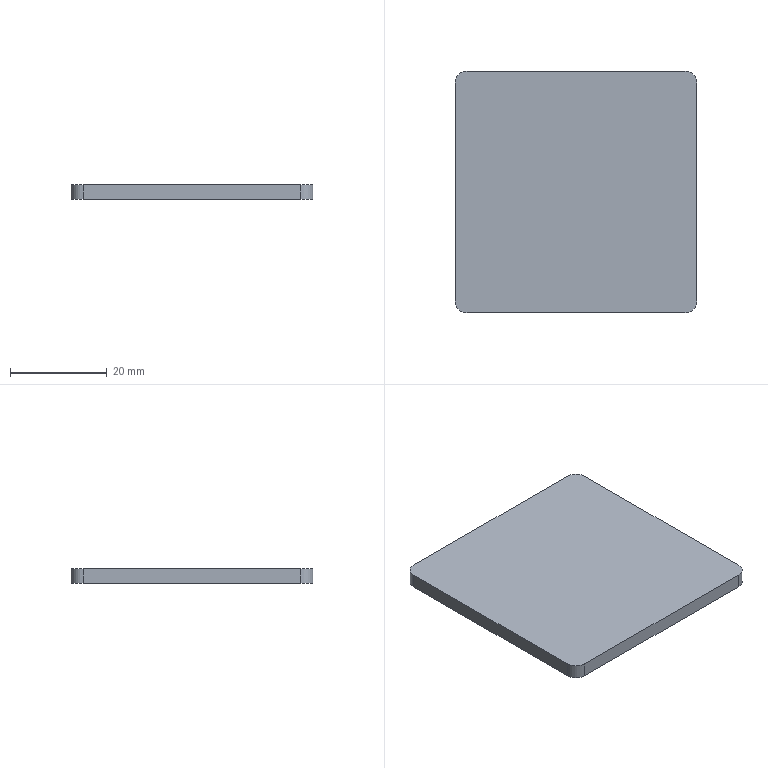Part | STEP file | 6100518 | 1 solid | 10 faces | box 50 x 50 x 3 mm | volume 7484 mm3 | plane 6 | cylinder 4 | commonest cylinder face diameters 5 x4
STEP:
#1=CARTESIAN_POINT('',(0.,0.,0.));
#2=DIRECTION('',(0.,0.,1.));
#3=DIRECTION('',(1.,0.,0.));
#4=AXIS2_PLACEMENT_3D('',#1,#2,#3);
#5=CARTESIAN_POINT('',(22.5,-25.,0.));
#6=VERTEX_POINT('',#5);
#7=CARTESIAN_POINT('',(25.,-22.5,0.));
#8=VERTEX_POINT('',#7);
#9=CARTESIAN_POINT('',(22.5,-22.5,0.));
#10=DIRECTION('',(0.,0.,1.));
#11=DIRECTION('',(1.,0.,0.));
#12=AXIS2_PLACEMENT_3D('',#9,#10,#11);
#13=CIRCLE('',#12,2.5);
#14=CARTESIAN_POINT('',(22.5,-22.5,3.));
#15=DIRECTION('',(0.,0.,-1.));
#16=DIRECTION('',(-1.,0.,0.));
#17=AXIS2_PLACEMENT_3D('',#14,#15,#16);
#18=CYLINDRICAL_SURFACE('',#17,2.5);
#19=CARTESIAN_POINT('',(9.425,3.));
#20=DIRECTION('',(-1.,0.));
#21=VECTOR('',#20,1.);
#22=LINE('',#19,#21);
#23=(GEOMETRIC_REPRESENTATION_CONTEXT(2)PARAMETRIC_REPRESENTATION_CONTEXT()REPRESENTATION_CONTEXT('',''));
#24=DEFINITIONAL_REPRESENTATION('',(#22),#23);
#25=PCURVE('',#18,#24);
#26=CARTESIAN_POINT('',(22.5,-22.5,0.));
#27=DIRECTION('',(0.,0.,1.));
#28=DIRECTION('',(1.,0.,0.));
#29=AXIS2_PLACEMENT_3D('',#26,#27,#28);
#30=PLANE('',#29);
#31=CARTESIAN_POINT('',(0.,0.));
#32=DIRECTION('',(1.,0.));
#33=AXIS2_PLACEMENT_2D('',#31,#32);
#34=CIRCLE('',#33,2.5);
#35=(GEOMETRIC_REPRESENTATION_CONTEXT(2)PARAMETRIC_REPRESENTATION_CONTEXT()REPRESENTATION_CONTEXT('',''));
#36=DEFINITIONAL_REPRESENTATION('',(#34),#35);
#37=PCURVE('',#30,#36);
#38=SURFACE_CURVE('',#13,(#25,#37),.PCURVE_S1.);
#39=EDGE_CURVE('',#6,#8,#38,.T.);
#40=ORIENTED_EDGE('',*,*,#39,.T.);
#41=CARTESIAN_POINT('',(25.,-22.5,3.));
#42=VERTEX_POINT('',#41);
#43=CARTESIAN_POINT('',(25.,-22.5,3.));
#44=DIRECTION('',(0.,0.,-1.));
#45=VECTOR('',#44,1.);
#46=LINE('',#43,#45);
#47=CARTESIAN_POINT('',(3.142,0.));
#48=DIRECTION('',(0.,1.));
#49=VECTOR('',#48,1.);
#50=LINE('',#47,#49);
#51=(GEOMETRIC_REPRESENTATION_CONTEXT(2)PARAMETRIC_REPRESENTATION_CONTEXT()REPRESENTATION_CONTEXT('',''));
#52=DEFINITIONAL_REPRESENTATION('',(#50),#51);
#53=PCURVE('',#18,#52);
#54=CARTESIAN_POINT('',(25.,22.5,3.));
#55=DIRECTION('',(-1.,0.,0.));
#56=DIRECTION('',(0.,-1.,0.));
#57=AXIS2_PLACEMENT_3D('',#54,#55,#56);
#58=PLANE('',#57);
#59=CARTESIAN_POINT('',(45.,0.));
#60=DIRECTION('',(0.,-1.));
#61=VECTOR('',#60,1.);
#62=LINE('',#59,#61);
#63=(GEOMETRIC_REPRESENTATION_CONTEXT(2)PARAMETRIC_REPRESENTATION_CONTEXT()REPRESENTATION_CONTEXT('',''));
#64=DEFINITIONAL_REPRESENTATION('',(#62),#63);
#65=PCURVE('',#58,#64);
#66=SURFACE_CURVE('',#46,(#53,#65),.PCURVE_S1.);
#67=EDGE_CURVE('',#42,#8,#66,.T.);
#68=ORIENTED_EDGE('',*,*,#67,.F.);
#69=CARTESIAN_POINT('',(22.5,-25.,3.));
#70=VERTEX_POINT('',#69);
#71=CARTESIAN_POINT('',(22.5,-22.5,3.));
#72=DIRECTION('',(0.,0.,1.));
#73=DIRECTION('',(1.,0.,0.));
#74=AXIS2_PLACEMENT_3D('',#71,#72,#73);
#75=CIRCLE('',#74,2.5);
#76=CARTESIAN_POINT('',(9.425,0.));
#77=DIRECTION('',(-1.,0.));
#78=VECTOR('',#77,1.);
#79=LINE('',#76,#78);
#80=(GEOMETRIC_REPRESENTATION_CONTEXT(2)PARAMETRIC_REPRESENTATION_CONTEXT()REPRESENTATION_CONTEXT('',''));
#81=DEFINITIONAL_REPRESENTATION('',(#79),#80);
#82=PCURVE('',#18,#81);
#83=CARTESIAN_POINT('',(22.5,-22.5,3.));
#84=DIRECTION('',(0.,0.,1.));
#85=DIRECTION('',(1.,0.,0.));
#86=AXIS2_PLACEMENT_3D('',#83,#84,#85);
#87=PLANE('',#86);
#88=CARTESIAN_POINT('',(0.,0.));
#89=DIRECTION('',(1.,0.));
#90=AXIS2_PLACEMENT_2D('',#88,#89);
#91=CIRCLE('',#90,2.5);
#92=(GEOMETRIC_REPRESENTATION_CONTEXT(2)PARAMETRIC_REPRESENTATION_CONTEXT()REPRESENTATION_CONTEXT('',''));
#93=DEFINITIONAL_REPRESENTATION('',(#91),#92);
#94=PCURVE('',#87,#93);
#95=SURFACE_CURVE('',#75,(#82,#94),.PCURVE_S1.);
#96=EDGE_CURVE('',#70,#42,#95,.T.);
#97=ORIENTED_EDGE('',*,*,#96,.F.);
#98=CARTESIAN_POINT('',(22.5,-25.,3.));
#99=DIRECTION('',(0.,0.,-1.));
#100=VECTOR('',#99,1.);
#101=LINE('',#98,#100);
#102=CARTESIAN_POINT('',(4.712,0.));
#103=DIRECTION('',(0.,1.));
#104=VECTOR('',#103,1.);
#105=LINE('',#102,#104);
#106=(GEOMETRIC_REPRESENTATION_CONTEXT(2)PARAMETRIC_REPRESENTATION_CONTEXT()REPRESENTATION_CONTEXT('',''));
#107=DEFINITIONAL_REPRESENTATION('',(#105),#106);
#108=PCURVE('',#18,#107);
#109=CARTESIAN_POINT('',(-22.5,-25.,3.));
#110=DIRECTION('',(0.,1.,0.));
#111=DIRECTION('',(-1.,0.,0.));
#112=AXIS2_PLACEMENT_3D('',#109,#110,#111);
#113=PLANE('',#112);
#114=CARTESIAN_POINT('',(-45.,0.));
#115=DIRECTION('',(0.,-1.));
#116=VECTOR('',#115,1.);
#117=LINE('',#114,#116);
#118=(GEOMETRIC_REPRESENTATION_CONTEXT(2)PARAMETRIC_REPRESENTATION_CONTEXT()REPRESENTATION_CONTEXT('',''));
#119=DEFINITIONAL_REPRESENTATION('',(#117),#118);
#120=PCURVE('',#113,#119);
#121=SURFACE_CURVE('',#101,(#108,#120),.PCURVE_S1.);
#122=EDGE_CURVE('',#70,#6,#121,.T.);
#123=ORIENTED_EDGE('',*,*,#122,.T.);
#124=EDGE_LOOP('',(#40,#68,#97,#123));
#125=FACE_BOUND('',#124,.T.);
#126=ADVANCED_FACE('',(#125),#18,.T.);
#127=CARTESIAN_POINT('',(25.,22.5,0.));
#128=VERTEX_POINT('',#127);
#129=CARTESIAN_POINT('',(25.,22.5,0.));
#130=DIRECTION('',(0.,1.,0.));
#131=VECTOR('',#130,1.);
#132=LINE('',#129,#131);
#133=CARTESIAN_POINT('',(0.,-3.));
#134=DIRECTION('',(-1.,0.));
#135=VECTOR('',#134,1.);
#136=LINE('',#133,#135);
#137=(GEOMETRIC_REPRESENTATION_CONTEXT(2)PARAMETRIC_REPRESENTATION_CONTEXT()REPRESENTATION_CONTEXT('',''));
#138=DEFINITIONAL_REPRESENTATION('',(#136),#137);
#139=PCURVE('',#58,#138);
#140=CARTESIAN_POINT('',(2.5,45.));
#141=DIRECTION('',(0.,1.));
#142=VECTOR('',#141,1.);
#143=LINE('',#140,#142);
#144=(GEOMETRIC_REPRESENTATION_CONTEXT(2)PARAMETRIC_REPRESENTATION_CONTEXT()REPRESENTATION_CONTEXT('',''));
#145=DEFINITIONAL_REPRESENTATION('',(#143),#144);
#146=PCURVE('',#30,#145);
#147=SURFACE_CURVE('',#132,(#139,#146),.PCURVE_S1.);
#148=EDGE_CURVE('',#8,#128,#147,.T.);
#149=ORIENTED_EDGE('',*,*,#148,.T.);
#150=CARTESIAN_POINT('',(25.,22.5,3.));
#151=VERTEX_POINT('',#150);
#152=CARTESIAN_POINT('',(25.,22.5,3.));
#153=DIRECTION('',(0.,0.,-1.));
#154=VECTOR('',#153,1.);
#155=LINE('',#152,#154);
#156=CARTESIAN_POINT('',(0.,0.));
#157=DIRECTION('',(0.,-1.));
#158=VECTOR('',#157,1.);
#159=LINE('',#156,#158);
#160=(GEOMETRIC_REPRESENTATION_CONTEXT(2)PARAMETRIC_REPRESENTATION_CONTEXT()REPRESENTATION_CONTEXT('',''));
#161=DEFINITIONAL_REPRESENTATION('',(#159),#160);
#162=PCURVE('',#58,#161);
#163=CARTESIAN_POINT('',(22.5,22.5,3.));
#164=DIRECTION('',(0.,0.,-1.));
#165=DIRECTION('',(-1.,0.,0.));
#166=AXIS2_PLACEMENT_3D('',#163,#164,#165);
#167=CYLINDRICAL_SURFACE('',#166,2.5);
#168=CARTESIAN_POINT('',(3.142,0.));
#169=DIRECTION('',(0.,1.));
#170=VECTOR('',#169,1.);
#171=LINE('',#168,#170);
#172=(GEOMETRIC_REPRESENTATION_CONTEXT(2)PARAMETRIC_REPRESENTATION_CONTEXT()REPRESENTATION_CONTEXT('',''));
#173=DEFINITIONAL_REPRESENTATION('',(#171),#172);
#174=PCURVE('',#167,#173);
#175=SURFACE_CURVE('',#155,(#162,#174),.PCURVE_S1.);
#176=EDGE_CURVE('',#151,#128,#175,.T.);
#177=ORIENTED_EDGE('',*,*,#176,.F.);
#178=CARTESIAN_POINT('',(25.,22.5,3.));
#179=DIRECTION('',(0.,1.,0.));
#180=VECTOR('',#179,1.);
#181=LINE('',#178,#180);
#182=CARTESIAN_POINT('',(0.,0.));
#183=DIRECTION('',(-1.,0.));
#184=VECTOR('',#183,1.);
#185=LINE('',#182,#184);
#186=(GEOMETRIC_REPRESENTATION_CONTEXT(2)PARAMETRIC_REPRESENTATION_CONTEXT()REPRESENTATION_CONTEXT('',''));
#187=DEFINITIONAL_REPRESENTATION('',(#185),#186);
#188=PCURVE('',#58,#187);
#189=CARTESIAN_POINT('',(2.5,45.));
#190=DIRECTION('',(0.,1.));
#191=VECTOR('',#190,1.);
#192=LINE('',#189,#191);
#193=(GEOMETRIC_REPRESENTATION_CONTEXT(2)PARAMETRIC_REPRESENTATION_CONTEXT()REPRESENTATION_CONTEXT('',''));
#194=DEFINITIONAL_REPRESENTATION('',(#192),#193);
#195=PCURVE('',#87,#194);
#196=SURFACE_CURVE('',#181,(#188,#195),.PCURVE_S1.);
#197=EDGE_CURVE('',#42,#151,#196,.T.);
#198=ORIENTED_EDGE('',*,*,#197,.F.);
#199=ORIENTED_EDGE('',*,*,#67,.T.);
#200=EDGE_LOOP('',(#149,#177,#198,#199));
#201=FACE_BOUND('',#200,.T.);
#202=ADVANCED_FACE('',(#201),#58,.F.);
#203=CARTESIAN_POINT('',(22.5,25.,0.));
#204=VERTEX_POINT('',#203);
#205=CARTESIAN_POINT('',(22.5,22.5,0.));
#206=DIRECTION('',(0.,0.,1.));
#207=DIRECTION('',(-1.,0.,0.));
#208=AXIS2_PLACEMENT_3D('',#205,#206,#207);
#209=CIRCLE('',#208,2.5);
#210=CARTESIAN_POINT('',(6.283,3.));
#211=DIRECTION('',(-1.,0.));
#212=VECTOR('',#211,1.);
#213=LINE('',#210,#212);
#214=(GEOMETRIC_REPRESENTATION_CONTEXT(2)PARAMETRIC_REPRESENTATION_CONTEXT()REPRESENTATION_CONTEXT('',''));
#215=DEFINITIONAL_REPRESENTATION('',(#213),#214);
#216=PCURVE('',#167,#215);
#217=CARTESIAN_POINT('',(0.,45.));
#218=DIRECTION('',(-1.,0.));
#219=AXIS2_PLACEMENT_2D('',#217,#218);
#220=CIRCLE('',#219,2.5);
#221=(GEOMETRIC_REPRESENTATION_CONTEXT(2)PARAMETRIC_REPRESENTATION_CONTEXT()REPRESENTATION_CONTEXT('',''));
#222=DEFINITIONAL_REPRESENTATION('',(#220),#221);
#223=PCURVE('',#30,#222);
#224=SURFACE_CURVE('',#209,(#216,#223),.PCURVE_S1.);
#225=EDGE_CURVE('',#128,#204,#224,.T.);
#226=ORIENTED_EDGE('',*,*,#225,.T.);
#227=CARTESIAN_POINT('',(22.5,25.,3.));
#228=VERTEX_POINT('',#227);
#229=CARTESIAN_POINT('',(22.5,25.,3.));
#230=DIRECTION('',(0.,0.,-1.));
#231=VECTOR('',#230,1.);
#232=LINE('',#229,#231);
#233=CARTESIAN_POINT('',(1.571,0.));
#234=DIRECTION('',(0.,1.));
#235=VECTOR('',#234,1.);
#236=LINE('',#233,#235);
#237=(GEOMETRIC_REPRESENTATION_CONTEXT(2)PARAMETRIC_REPRESENTATION_CONTEXT()REPRESENTATION_CONTEXT('',''));
#238=DEFINITIONAL_REPRESENTATION('',(#236),#237);
#239=PCURVE('',#167,#238);
#240=CARTESIAN_POINT('',(-22.5,25.,3.));
#241=DIRECTION('',(0.,-1.,0.));
#242=DIRECTION('',(0.,0.,-1.));
#243=AXIS2_PLACEMENT_3D('',#240,#241,#242);
#244=PLANE('',#243);
#245=CARTESIAN_POINT('',(0.,45.));
#246=DIRECTION('',(1.,0.));
#247=VECTOR('',#246,1.);
#248=LINE('',#245,#247);
#249=(GEOMETRIC_REPRESENTATION_CONTEXT(2)PARAMETRIC_REPRESENTATION_CONTEXT()REPRESENTATION_CONTEXT('',''));
#250=DEFINITIONAL_REPRESENTATION('',(#248),#249);
#251=PCURVE('',#244,#250);
#252=SURFACE_CURVE('',#232,(#239,#251),.PCURVE_S1.);
#253=EDGE_CURVE('',#228,#204,#252,.T.);
#254=ORIENTED_EDGE('',*,*,#253,.F.);
#255=CARTESIAN_POINT('',(22.5,22.5,3.));
#256=DIRECTION('',(0.,0.,1.));
#257=DIRECTION('',(-1.,0.,0.));
#258=AXIS2_PLACEMENT_3D('',#255,#256,#257);
#259=CIRCLE('',#258,2.5);
#260=CARTESIAN_POINT('',(6.283,0.));
#261=DIRECTION('',(-1.,0.));
#262=VECTOR('',#261,1.);
#263=LINE('',#260,#262);
#264=(GEOMETRIC_REPRESENTATION_CONTEXT(2)PARAMETRIC_REPRESENTATION_CONTEXT()REPRESENTATION_CONTEXT('',''));
#265=DEFINITIONAL_REPRESENTATION('',(#263),#264);
#266=PCURVE('',#167,#265);
#267=CARTESIAN_POINT('',(0.,45.));
#268=DIRECTION('',(-1.,0.));
#269=AXIS2_PLACEMENT_2D('',#267,#268);
#270=CIRCLE('',#269,2.5);
#271=(GEOMETRIC_REPRESENTATION_CONTEXT(2)PARAMETRIC_REPRESENTATION_CONTEXT()REPRESENTATION_CONTEXT('',''));
#272=DEFINITIONAL_REPRESENTATION('',(#270),#271);
#273=PCURVE('',#87,#272);
#274=SURFACE_CURVE('',#259,(#266,#273),.PCURVE_S1.);
#275=EDGE_CURVE('',#151,#228,#274,.T.);
#276=ORIENTED_EDGE('',*,*,#275,.F.);
#277=ORIENTED_EDGE('',*,*,#176,.T.);
#278=EDGE_LOOP('',(#226,#254,#276,#277));
#279=FACE_BOUND('',#278,.T.);
#280=ADVANCED_FACE('',(#279),#167,.T.);
#281=CARTESIAN_POINT('',(-22.5,25.,0.));
#282=VERTEX_POINT('',#281);
#283=CARTESIAN_POINT('',(-22.5,25.,0.));
#284=DIRECTION('',(-1.,0.,0.));
#285=VECTOR('',#284,1.);
#286=LINE('',#283,#285);
#287=CARTESIAN_POINT('',(3.,0.));
#288=DIRECTION('',(0.,-1.));
#289=VECTOR('',#288,1.);
#290=LINE('',#287,#289);
#291=(GEOMETRIC_REPRESENTATION_CONTEXT(2)PARAMETRIC_REPRESENTATION_CONTEXT()REPRESENTATION_CONTEXT('',''));
#292=DEFINITIONAL_REPRESENTATION('',(#290),#291);
#293=PCURVE('',#244,#292);
#294=CARTESIAN_POINT('',(-45.,47.5));
#295=DIRECTION('',(-1.,0.));
#296=VECTOR('',#295,1.);
#297=LINE('',#294,#296);
#298=(GEOMETRIC_REPRESENTATION_CONTEXT(2)PARAMETRIC_REPRESENTATION_CONTEXT()REPRESENTATION_CONTEXT('',''));
#299=DEFINITIONAL_REPRESENTATION('',(#297),#298);
#300=PCURVE('',#30,#299);
#301=SURFACE_CURVE('',#286,(#293,#300),.PCURVE_S1.);
#302=EDGE_CURVE('',#204,#282,#301,.T.);
#303=ORIENTED_EDGE('',*,*,#302,.T.);
#304=CARTESIAN_POINT('',(-22.5,25.,3.));
#305=VERTEX_POINT('',#304);
#306=CARTESIAN_POINT('',(-22.5,25.,3.));
#307=DIRECTION('',(0.,0.,-1.));
#308=VECTOR('',#307,1.);
#309=LINE('',#306,#308);
#310=CARTESIAN_POINT('',(0.,0.));
#311=DIRECTION('',(1.,0.));
#312=VECTOR('',#311,1.);
#313=LINE('',#310,#312);
#314=(GEOMETRIC_REPRESENTATION_CONTEXT(2)PARAMETRIC_REPRESENTATION_CONTEXT()REPRESENTATION_CONTEXT('',''));
#315=DEFINITIONAL_REPRESENTATION('',(#313),#314);
#316=PCURVE('',#244,#315);
#317=CARTESIAN_POINT('',(-22.5,22.5,3.));
#318=DIRECTION('',(0.,0.,-1.));
#319=DIRECTION('',(-1.,0.,0.));
#320=AXIS2_PLACEMENT_3D('',#317,#318,#319);
#321=CYLINDRICAL_SURFACE('',#320,2.5);
#322=CARTESIAN_POINT('',(1.571,0.));
#323=DIRECTION('',(0.,1.));
#324=VECTOR('',#323,1.);
#325=LINE('',#322,#324);
#326=(GEOMETRIC_REPRESENTATION_CONTEXT(2)PARAMETRIC_REPRESENTATION_CONTEXT()REPRESENTATION_CONTEXT('',''));
#327=DEFINITIONAL_REPRESENTATION('',(#325),#326);
#328=PCURVE('',#321,#327);
#329=SURFACE_CURVE('',#309,(#316,#328),.PCURVE_S1.);
#330=EDGE_CURVE('',#305,#282,#329,.T.);
#331=ORIENTED_EDGE('',*,*,#330,.F.);
#332=CARTESIAN_POINT('',(-22.5,25.,3.));
#333=DIRECTION('',(-1.,0.,0.));
#334=VECTOR('',#333,1.);
#335=LINE('',#332,#334);
#336=CARTESIAN_POINT('',(0.,0.));
#337=DIRECTION('',(0.,-1.));
#338=VECTOR('',#337,1.);
#339=LINE('',#336,#338);
#340=(GEOMETRIC_REPRESENTATION_CONTEXT(2)PARAMETRIC_REPRESENTATION_CONTEXT()REPRESENTATION_CONTEXT('',''));
#341=DEFINITIONAL_REPRESENTATION('',(#339),#340);
#342=PCURVE('',#244,#341);
#343=CARTESIAN_POINT('',(-45.,47.5));
#344=DIRECTION('',(-1.,0.));
#345=VECTOR('',#344,1.);
#346=LINE('',#343,#345);
#347=(GEOMETRIC_REPRESENTATION_CONTEXT(2)PARAMETRIC_REPRESENTATION_CONTEXT()REPRESENTATION_CONTEXT('',''));
#348=DEFINITIONAL_REPRESENTATION('',(#346),#347);
#349=PCURVE('',#87,#348);
#350=SURFACE_CURVE('',#335,(#342,#349),.PCURVE_S1.);
#351=EDGE_CURVE('',#228,#305,#350,.T.);
#352=ORIENTED_EDGE('',*,*,#351,.F.);
#353=ORIENTED_EDGE('',*,*,#253,.T.);
#354=EDGE_LOOP('',(#303,#331,#352,#353));
#355=FACE_BOUND('',#354,.T.);
#356=ADVANCED_FACE('',(#355),#244,.F.);
#357=CARTESIAN_POINT('',(-25.,22.5,0.));
#358=VERTEX_POINT('',#357);
#359=CARTESIAN_POINT('',(-22.5,22.5,0.));
#360=DIRECTION('',(0.,0.,1.));
#361=DIRECTION('',(1.,0.,0.));
#362=AXIS2_PLACEMENT_3D('',#359,#360,#361);
#363=CIRCLE('',#362,2.5);
#364=CARTESIAN_POINT('',(3.142,3.));
#365=DIRECTION('',(-1.,0.));
#366=VECTOR('',#365,1.);
#367=LINE('',#364,#366);
#368=(GEOMETRIC_REPRESENTATION_CONTEXT(2)PARAMETRIC_REPRESENTATION_CONTEXT()REPRESENTATION_CONTEXT('',''));
#369=DEFINITIONAL_REPRESENTATION('',(#367),#368);
#370=PCURVE('',#321,#369);
#371=CARTESIAN_POINT('',(-45.,45.));
#372=DIRECTION('',(1.,0.));
#373=AXIS2_PLACEMENT_2D('',#371,#372);
#374=CIRCLE('',#373,2.5);
#375=(GEOMETRIC_REPRESENTATION_CONTEXT(2)PARAMETRIC_REPRESENTATION_CONTEXT()REPRESENTATION_CONTEXT('',''));
#376=DEFINITIONAL_REPRESENTATION('',(#374),#375);
#377=PCURVE('',#30,#376);
#378=SURFACE_CURVE('',#363,(#370,#377),.PCURVE_S1.);
#379=EDGE_CURVE('',#282,#358,#378,.T.);
#380=ORIENTED_EDGE('',*,*,#379,.T.);
#381=CARTESIAN_POINT('',(-25.,22.5,3.));
#382=VERTEX_POINT('',#381);
#383=CARTESIAN_POINT('',(-25.,22.5,3.));
#384=DIRECTION('',(0.,0.,-1.));
#385=VECTOR('',#384,1.);
#386=LINE('',#383,#385);
#387=CARTESIAN_POINT('',(0.,0.));
#388=DIRECTION('',(0.,1.));
#389=VECTOR('',#388,1.);
#390=LINE('',#387,#389);
#391=(GEOMETRIC_REPRESENTATION_CONTEXT(2)PARAMETRIC_REPRESENTATION_CONTEXT()REPRESENTATION_CONTEXT('',''));
#392=DEFINITIONAL_REPRESENTATION('',(#390),#391);
#393=PCURVE('',#321,#392);
#394=CARTESIAN_POINT('',(-25.,22.5,3.));
#395=DIRECTION('',(1.,0.,0.));
#396=DIRECTION('',(0.,1.,0.));
#397=AXIS2_PLACEMENT_3D('',#394,#395,#396);
#398=PLANE('',#397);
#399=CARTESIAN_POINT('',(0.,0.));
#400=DIRECTION('',(0.,-1.));
#401=VECTOR('',#400,1.);
#402=LINE('',#399,#401);
#403=(GEOMETRIC_REPRESENTATION_CONTEXT(2)PARAMETRIC_REPRESENTATION_CONTEXT()REPRESENTATION_CONTEXT('',''));
#404=DEFINITIONAL_REPRESENTATION('',(#402),#403);
#405=PCURVE('',#398,#404);
#406=SURFACE_CURVE('',#386,(#393,#405),.PCURVE_S1.);
#407=EDGE_CURVE('',#382,#358,#406,.T.);
#408=ORIENTED_EDGE('',*,*,#407,.F.);
#409=CARTESIAN_POINT('',(-22.5,22.5,3.));
#410=DIRECTION('',(0.,0.,1.));
#411=DIRECTION('',(1.,0.,0.));
#412=AXIS2_PLACEMENT_3D('',#409,#410,#411);
#413=CIRCLE('',#412,2.5);
#414=CARTESIAN_POINT('',(3.142,0.));
#415=DIRECTION('',(-1.,0.));
#416=VECTOR('',#415,1.);
#417=LINE('',#414,#416);
#418=(GEOMETRIC_REPRESENTATION_CONTEXT(2)PARAMETRIC_REPRESENTATION_CONTEXT()REPRESENTATION_CONTEXT('',''));
#419=DEFINITIONAL_REPRESENTATION('',(#417),#418);
#420=PCURVE('',#321,#419);
#421=CARTESIAN_POINT('',(-45.,45.));
#422=DIRECTION('',(1.,0.));
#423=AXIS2_PLACEMENT_2D('',#421,#422);
#424=CIRCLE('',#423,2.5);
#425=(GEOMETRIC_REPRESENTATION_CONTEXT(2)PARAMETRIC_REPRESENTATION_CONTEXT()REPRESENTATION_CONTEXT('',''));
#426=DEFINITIONAL_REPRESENTATION('',(#424),#425);
#427=PCURVE('',#87,#426);
#428=SURFACE_CURVE('',#413,(#420,#427),.PCURVE_S1.);
#429=EDGE_CURVE('',#305,#382,#428,.T.);
#430=ORIENTED_EDGE('',*,*,#429,.F.);
#431=ORIENTED_EDGE('',*,*,#330,.T.);
#432=EDGE_LOOP('',(#380,#408,#430,#431));
#433=FACE_BOUND('',#432,.T.);
#434=ADVANCED_FACE('',(#433),#321,.T.);
#435=CARTESIAN_POINT('',(-25.,-22.5,0.));
#436=VERTEX_POINT('',#435);
#437=CARTESIAN_POINT('',(-25.,22.5,0.));
#438=DIRECTION('',(0.,-1.,0.));
#439=VECTOR('',#438,1.);
#440=LINE('',#437,#439);
#441=CARTESIAN_POINT('',(0.,-3.));
#442=DIRECTION('',(-1.,0.));
#443=VECTOR('',#442,1.);
#444=LINE('',#441,#443);
#445=(GEOMETRIC_REPRESENTATION_CONTEXT(2)PARAMETRIC_REPRESENTATION_CONTEXT()REPRESENTATION_CONTEXT('',''));
#446=DEFINITIONAL_REPRESENTATION('',(#444),#445);
#447=PCURVE('',#398,#446);
#448=CARTESIAN_POINT('',(-47.5,45.));
#449=DIRECTION('',(0.,-1.));
#450=VECTOR('',#449,1.);
#451=LINE('',#448,#450);
#452=(GEOMETRIC_REPRESENTATION_CONTEXT(2)PARAMETRIC_REPRESENTATION_CONTEXT()REPRESENTATION_CONTEXT('',''));
#453=DEFINITIONAL_REPRESENTATION('',(#451),#452);
#454=PCURVE('',#30,#453);
#455=SURFACE_CURVE('',#440,(#447,#454),.PCURVE_S1.);
#456=EDGE_CURVE('',#358,#436,#455,.T.);
#457=ORIENTED_EDGE('',*,*,#456,.T.);
#458=CARTESIAN_POINT('',(-25.,-22.5,3.));
#459=VERTEX_POINT('',#458);
#460=CARTESIAN_POINT('',(-25.,-22.5,3.));
#461=DIRECTION('',(0.,0.,-1.));
#462=VECTOR('',#461,1.);
#463=LINE('',#460,#462);
#464=CARTESIAN_POINT('',(-45.,0.));
#465=DIRECTION('',(0.,-1.));
#466=VECTOR('',#465,1.);
#467=LINE('',#464,#466);
#468=(GEOMETRIC_REPRESENTATION_CONTEXT(2)PARAMETRIC_REPRESENTATION_CONTEXT()REPRESENTATION_CONTEXT('',''));
#469=DEFINITIONAL_REPRESENTATION('',(#467),#468);
#470=PCURVE('',#398,#469);
#471=CARTESIAN_POINT('',(-22.5,-22.5,3.));
#472=DIRECTION('',(0.,0.,-1.));
#473=DIRECTION('',(-1.,0.,0.));
#474=AXIS2_PLACEMENT_3D('',#471,#472,#473);
#475=CYLINDRICAL_SURFACE('',#474,2.5);
#476=CARTESIAN_POINT('',(6.283,0.));
#477=DIRECTION('',(0.,1.));
#478=VECTOR('',#477,1.);
#479=LINE('',#476,#478);
#480=(GEOMETRIC_REPRESENTATION_CONTEXT(2)PARAMETRIC_REPRESENTATION_CONTEXT()REPRESENTATION_CONTEXT('',''));
#481=DEFINITIONAL_REPRESENTATION('',(#479),#480);
#482=PCURVE('',#475,#481);
#483=SURFACE_CURVE('',#463,(#470,#482),.PCURVE_S1.);
#484=EDGE_CURVE('',#459,#436,#483,.T.);
#485=ORIENTED_EDGE('',*,*,#484,.F.);
#486=CARTESIAN_POINT('',(-25.,22.5,3.));
#487=DIRECTION('',(0.,-1.,0.));
#488=VECTOR('',#487,1.);
#489=LINE('',#486,#488);
#490=CARTESIAN_POINT('',(0.,0.));
#491=DIRECTION('',(-1.,0.));
#492=VECTOR('',#491,1.);
#493=LINE('',#490,#492);
#494=(GEOMETRIC_REPRESENTATION_CONTEXT(2)PARAMETRIC_REPRESENTATION_CONTEXT()REPRESENTATION_CONTEXT('',''));
#495=DEFINITIONAL_REPRESENTATION('',(#493),#494);
#496=PCURVE('',#398,#495);
#497=CARTESIAN_POINT('',(-47.5,45.));
#498=DIRECTION('',(0.,-1.));
#499=VECTOR('',#498,1.);
#500=LINE('',#497,#499);
#501=(GEOMETRIC_REPRESENTATION_CONTEXT(2)PARAMETRIC_REPRESENTATION_CONTEXT()REPRESENTATION_CONTEXT('',''));
#502=DEFINITIONAL_REPRESENTATION('',(#500),#501);
#503=PCURVE('',#87,#502);
#504=SURFACE_CURVE('',#489,(#496,#503),.PCURVE_S1.);
#505=EDGE_CURVE('',#382,#459,#504,.T.);
#506=ORIENTED_EDGE('',*,*,#505,.F.);
#507=ORIENTED_EDGE('',*,*,#407,.T.);
#508=EDGE_LOOP('',(#457,#485,#506,#507));
#509=FACE_BOUND('',#508,.T.);
#510=ADVANCED_FACE('',(#509),#398,.F.);
#511=CARTESIAN_POINT('',(-22.5,-25.,0.));
#512=VERTEX_POINT('',#511);
#513=CARTESIAN_POINT('',(-22.5,-22.5,0.));
#514=DIRECTION('',(0.,0.,1.));
#515=DIRECTION('',(1.,0.,0.));
#516=AXIS2_PLACEMENT_3D('',#513,#514,#515);
#517=CIRCLE('',#516,2.5);
#518=CARTESIAN_POINT('',(9.425,3.));
#519=DIRECTION('',(-1.,0.));
#520=VECTOR('',#519,1.);
#521=LINE('',#518,#520);
#522=(GEOMETRIC_REPRESENTATION_CONTEXT(2)PARAMETRIC_REPRESENTATION_CONTEXT()REPRESENTATION_CONTEXT('',''));
#523=DEFINITIONAL_REPRESENTATION('',(#521),#522);
#524=PCURVE('',#475,#523);
#525=CARTESIAN_POINT('',(-45.,0.));
#526=DIRECTION('',(1.,0.));
#527=AXIS2_PLACEMENT_2D('',#525,#526);
#528=CIRCLE('',#527,2.5);
#529=(GEOMETRIC_REPRESENTATION_CONTEXT(2)PARAMETRIC_REPRESENTATION_CONTEXT()REPRESENTATION_CONTEXT('',''));
#530=DEFINITIONAL_REPRESENTATION('',(#528),#529);
#531=PCURVE('',#30,#530);
#532=SURFACE_CURVE('',#517,(#524,#531),.PCURVE_S1.);
#533=EDGE_CURVE('',#436,#512,#532,.T.);
#534=ORIENTED_EDGE('',*,*,#533,.T.);
#535=CARTESIAN_POINT('',(-22.5,-25.,3.));
#536=VERTEX_POINT('',#535);
#537=CARTESIAN_POINT('',(-22.5,-25.,3.));
#538=DIRECTION('',(0.,0.,-1.));
#539=VECTOR('',#538,1.);
#540=LINE('',#537,#539);
#541=CARTESIAN_POINT('',(4.712,0.));
#542=DIRECTION('',(0.,1.));
#543=VECTOR('',#542,1.);
#544=LINE('',#541,#543);
#545=(GEOMETRIC_REPRESENTATION_CONTEXT(2)PARAMETRIC_REPRESENTATION_CONTEXT()REPRESENTATION_CONTEXT('',''));
#546=DEFINITIONAL_REPRESENTATION('',(#544),#545);
#547=PCURVE('',#475,#546);
#548=CARTESIAN_POINT('',(0.,0.));
#549=DIRECTION('',(0.,-1.));
#550=VECTOR('',#549,1.);
#551=LINE('',#548,#550);
#552=(GEOMETRIC_REPRESENTATION_CONTEXT(2)PARAMETRIC_REPRESENTATION_CONTEXT()REPRESENTATION_CONTEXT('',''));
#553=DEFINITIONAL_REPRESENTATION('',(#551),#552);
#554=PCURVE('',#113,#553);
#555=SURFACE_CURVE('',#540,(#547,#554),.PCURVE_S1.);
#556=EDGE_CURVE('',#536,#512,#555,.T.);
#557=ORIENTED_EDGE('',*,*,#556,.F.);
#558=CARTESIAN_POINT('',(-22.5,-22.5,3.));
#559=DIRECTION('',(0.,0.,1.));
#560=DIRECTION('',(1.,0.,0.));
#561=AXIS2_PLACEMENT_3D('',#558,#559,#560);
#562=CIRCLE('',#561,2.5);
#563=CARTESIAN_POINT('',(9.425,0.));
#564=DIRECTION('',(-1.,0.));
#565=VECTOR('',#564,1.);
#566=LINE('',#563,#565);
#567=(GEOMETRIC_REPRESENTATION_CONTEXT(2)PARAMETRIC_REPRESENTATION_CONTEXT()REPRESENTATION_CONTEXT('',''));
#568=DEFINITIONAL_REPRESENTATION('',(#566),#567);
#569=PCURVE('',#475,#568);
#570=CARTESIAN_POINT('',(-45.,0.));
#571=DIRECTION('',(1.,0.));
#572=AXIS2_PLACEMENT_2D('',#570,#571);
#573=CIRCLE('',#572,2.5);
#574=(GEOMETRIC_REPRESENTATION_CONTEXT(2)PARAMETRIC_REPRESENTATION_CONTEXT()REPRESENTATION_CONTEXT('',''));
#575=DEFINITIONAL_REPRESENTATION('',(#573),#574);
#576=PCURVE('',#87,#575);
#577=SURFACE_CURVE('',#562,(#569,#576),.PCURVE_S1.);
#578=EDGE_CURVE('',#459,#536,#577,.T.);
#579=ORIENTED_EDGE('',*,*,#578,.F.);
#580=ORIENTED_EDGE('',*,*,#484,.T.);
#581=EDGE_LOOP('',(#534,#557,#579,#580));
#582=FACE_BOUND('',#581,.T.);
#583=ADVANCED_FACE('',(#582),#475,.T.);
#584=CARTESIAN_POINT('',(-22.5,-25.,0.));
#585=DIRECTION('',(1.,0.,0.));
#586=VECTOR('',#585,1.);
#587=LINE('',#584,#586);
#588=CARTESIAN_POINT('',(0.,-3.));
#589=DIRECTION('',(-1.,0.));
#590=VECTOR('',#589,1.);
#591=LINE('',#588,#590);
#592=(GEOMETRIC_REPRESENTATION_CONTEXT(2)PARAMETRIC_REPRESENTATION_CONTEXT()REPRESENTATION_CONTEXT('',''));
#593=DEFINITIONAL_REPRESENTATION('',(#591),#592);
#594=PCURVE('',#113,#593);
#595=CARTESIAN_POINT('',(-45.,-2.5));
#596=DIRECTION('',(1.,0.));
#597=VECTOR('',#596,1.);
#598=LINE('',#595,#597);
#599=(GEOMETRIC_REPRESENTATION_CONTEXT(2)PARAMETRIC_REPRESENTATION_CONTEXT()REPRESENTATION_CONTEXT('',''));
#600=DEFINITIONAL_REPRESENTATION('',(#598),#599);
#601=PCURVE('',#30,#600);
#602=SURFACE_CURVE('',#587,(#594,#601),.PCURVE_S1.);
#603=EDGE_CURVE('',#512,#6,#602,.T.);
#604=ORIENTED_EDGE('',*,*,#603,.T.);
#605=ORIENTED_EDGE('',*,*,#122,.F.);
#606=CARTESIAN_POINT('',(-22.5,-25.,3.));
#607=DIRECTION('',(1.,0.,0.));
#608=VECTOR('',#607,1.);
#609=LINE('',#606,#608);
#610=CARTESIAN_POINT('',(0.,0.));
#611=DIRECTION('',(-1.,0.));
#612=VECTOR('',#611,1.);
#613=LINE('',#610,#612);
#614=(GEOMETRIC_REPRESENTATION_CONTEXT(2)PARAMETRIC_REPRESENTATION_CONTEXT()REPRESENTATION_CONTEXT('',''));
#615=DEFINITIONAL_REPRESENTATION('',(#613),#614);
#616=PCURVE('',#113,#615);
#617=CARTESIAN_POINT('',(-45.,-2.5));
#618=DIRECTION('',(1.,0.));
#619=VECTOR('',#618,1.);
#620=LINE('',#617,#619);
#621=(GEOMETRIC_REPRESENTATION_CONTEXT(2)PARAMETRIC_REPRESENTATION_CONTEXT()REPRESENTATION_CONTEXT('',''));
#622=DEFINITIONAL_REPRESENTATION('',(#620),#621);
#623=PCURVE('',#87,#622);
#624=SURFACE_CURVE('',#609,(#616,#623),.PCURVE_S1.);
#625=EDGE_CURVE('',#536,#70,#624,.T.);
#626=ORIENTED_EDGE('',*,*,#625,.F.);
#627=ORIENTED_EDGE('',*,*,#556,.T.);
#628=EDGE_LOOP('',(#604,#605,#626,#627));
#629=FACE_BOUND('',#628,.T.);
#630=ADVANCED_FACE('',(#629),#113,.F.);
#631=ORIENTED_EDGE('',*,*,#96,.T.);
#632=ORIENTED_EDGE('',*,*,#197,.T.);
#633=ORIENTED_EDGE('',*,*,#275,.T.);
#634=ORIENTED_EDGE('',*,*,#351,.T.);
#635=ORIENTED_EDGE('',*,*,#429,.T.);
#636=ORIENTED_EDGE('',*,*,#505,.T.);
#637=ORIENTED_EDGE('',*,*,#578,.T.);
#638=ORIENTED_EDGE('',*,*,#625,.T.);
#639=EDGE_LOOP('',(#631,#632,#633,#634,#635,#636,#637,#638));
#640=FACE_BOUND('',#639,.T.);
#641=ADVANCED_FACE('',(#640),#87,.T.);
#642=ORIENTED_EDGE('',*,*,#39,.F.);
#643=ORIENTED_EDGE('',*,*,#603,.F.);
#644=ORIENTED_EDGE('',*,*,#533,.F.);
#645=ORIENTED_EDGE('',*,*,#456,.F.);
#646=ORIENTED_EDGE('',*,*,#379,.F.);
#647=ORIENTED_EDGE('',*,*,#302,.F.);
#648=ORIENTED_EDGE('',*,*,#225,.F.);
#649=ORIENTED_EDGE('',*,*,#148,.F.);
#650=EDGE_LOOP('',(#642,#643,#644,#645,#646,#647,#648,#649));
#651=FACE_BOUND('',#650,.T.);
#652=ADVANCED_FACE('',(#651),#30,.F.);
#653=CLOSED_SHELL('',(#126,#202,#280,#356,#434,#510,#583,#630,#641,#652));
#654=MANIFOLD_SOLID_BREP('',#653);
#655=(LENGTH_UNIT()NAMED_UNIT(*)SI_UNIT(.MILLI.,.METRE.));
#656=UNCERTAINTY_MEASURE_WITH_UNIT(LENGTH_MEASURE(0.0000001),#655,'','');
#657=(NAMED_UNIT(*)PLANE_ANGLE_UNIT()SI_UNIT($,.RADIAN.));
#658=(NAMED_UNIT(*)SI_UNIT($,.STERADIAN.)SOLID_ANGLE_UNIT());
#659=(GEOMETRIC_REPRESENTATION_CONTEXT(3)GLOBAL_UNCERTAINTY_ASSIGNED_CONTEXT((#656))GLOBAL_UNIT_ASSIGNED_CONTEXT((#655,#657,#658))REPRESENTATION_CONTEXT('',''));
#660=ADVANCED_BREP_SHAPE_REPRESENTATION('',(#4,#654),#659);